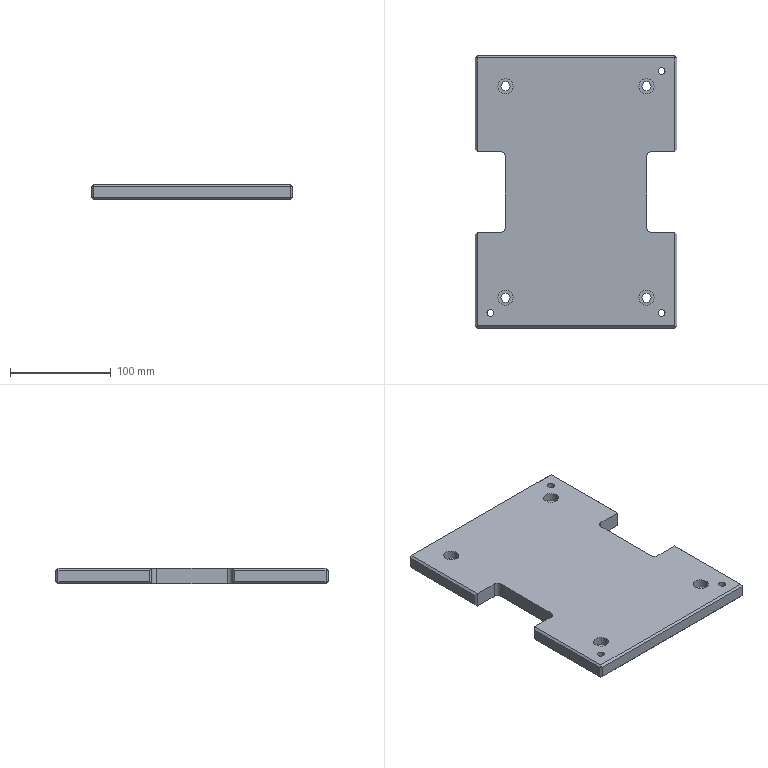Part | STEP file | Screw jig plate | 1 solid | 72 faces | box 200 x 270 x 15 mm | volume 725684 mm3 | plane 46 | cylinder 26 | commonest cylinder face diameters 9 x8 15 x8 6.8 x6 10 x4